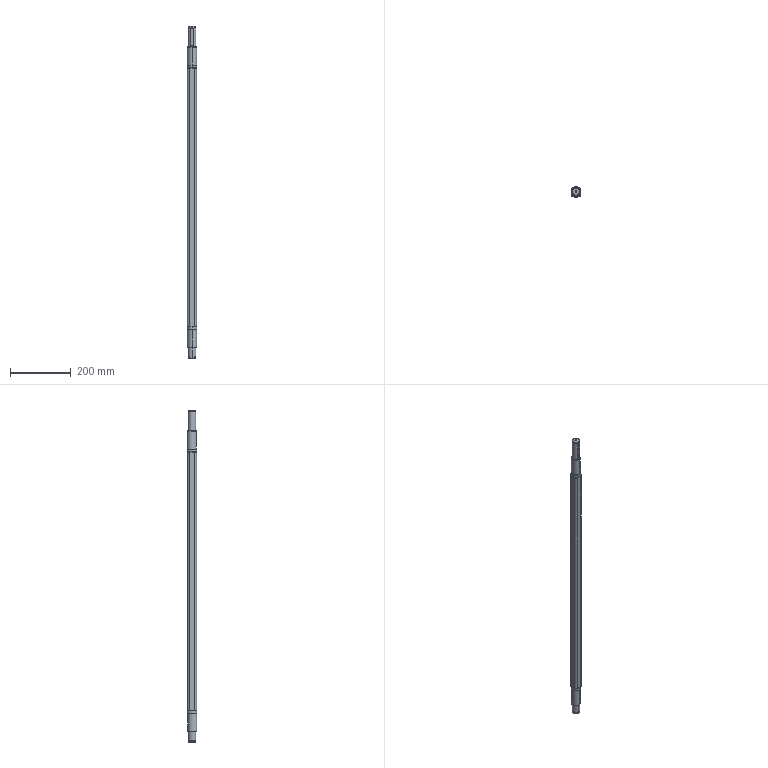Part | SolidWorks | features LayoutProfileFeature 1 | 8 solids | 155 faces | box 32 x 32.7 x 1096 mm | volume 415799 mm3 | cylinder 60 | plane 51 | cone 36 | spline 8 | commonest cylinder face diameters 15 x18 9 x12 25 x8 8 x4 23.5 x4 24 x4